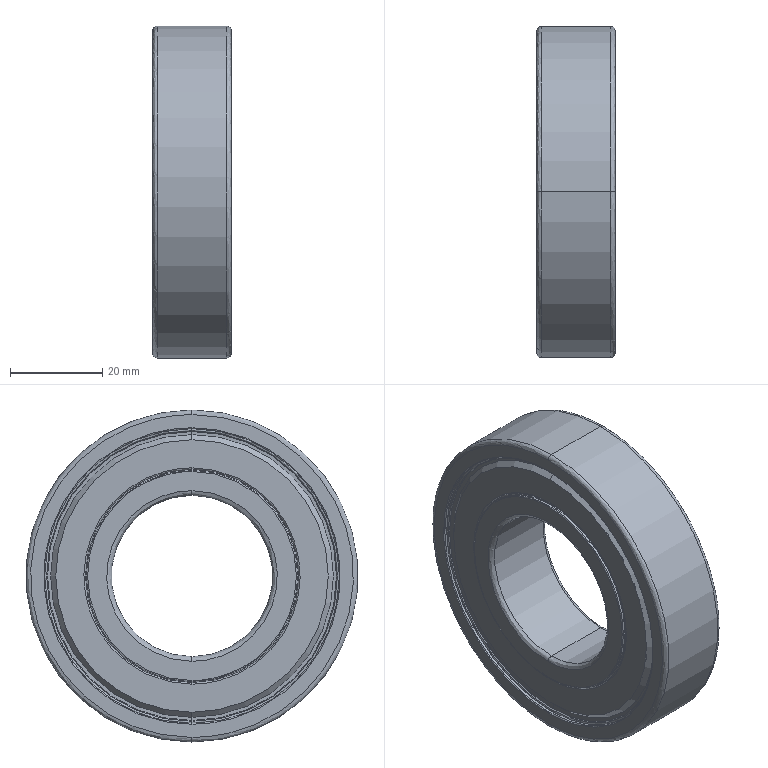Part | SolidWorks | features BaseBody 1 | 1 solid | 134 faces | box 17 x 72 x 72 mm | volume 43583 mm3 | spline 54 | cone 40 | cylinder 28 | plane 12 | commonest cylinder face diameters 45.7 x4 46.3 x4 46.9 x4 47.3 x4 61.7 x4 63.9 x4